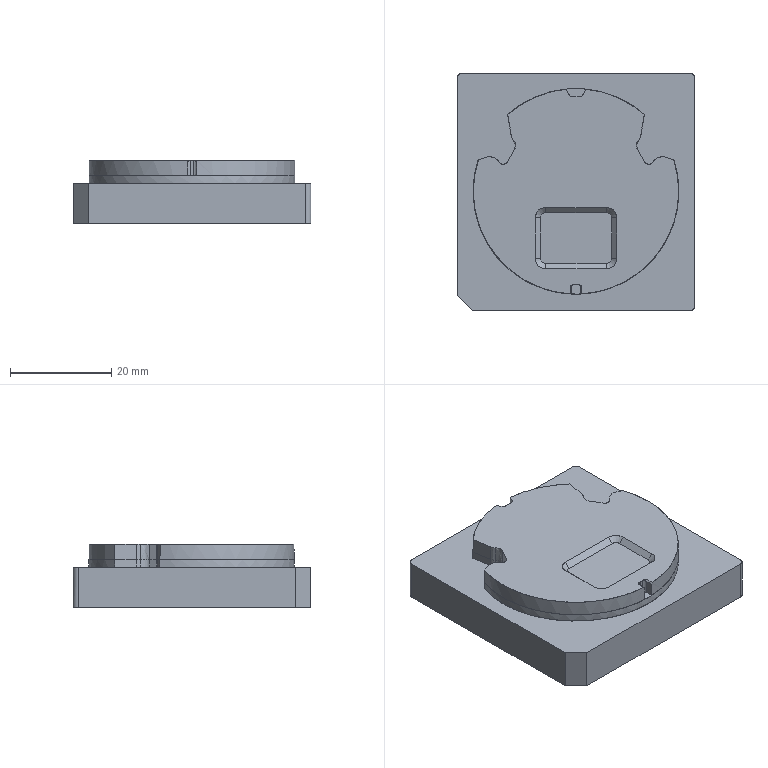NC program | PowerMill | posted with a generic post | part box 47 x 47 x 12.511 mm
Lines 1 to 1032 of 232111:
%
O0001
N104 ( POWERMILL CB  : 2026004.0)
N105 ( POST VER      : 2026.0.0.5161)
N106 ( OPTION FILE   : FANUC)
N107 ( OUTPUT WORKPLANE : WORLD)
N108 (  )
N109 ( TOOL LIST )
N110 (---------------------------------------)
N111 ( NO. | ID        | DIA.| TIP RAD|LENGTH)
N112 (---------------------------------------)
N113 (    1|D10C_1_1   |10.0 |  0.0   |67.96 )
N114 (   15|D3C_1_1    | 3.0 |  0.0   |59.56 )
N115 (   27|D1C_1_1    | 1.0 |  0.0   |59.72 )
N116 (    3|D10_1_1    |10.0 |  0.0   |67.68 )
N117 (   14|D4_1_1     | 4.0 |  0.0   |59.68 )
N118 (   12|D2_1       | 2.0 |  0.0   | 57.0 )
N119 (   12|D2_2_1     | 2.0 |  0.0   |59.68 )
N120 (    8|D1_1_1     | 1.0 |  0.0   |59.68 )
N121 (   13|TEXT_D4_1_1| 4.0 |  0.3   | 60.0 )
N122 (---------------------------------------)
N123 (  )
N124 ( NUMBER OF TOOLPATHS: 15.0 )
N125 ( ESTIMATED PROGRAM DURATION: 0 HOURS 23 MIN 32 SEC)
N126 (  )
N127 G00 G21 G80 G40 G17
N128 G90
N129 G54
N130 G53 Z0.0
N131 (---------------)
N132 ( START TOOLPATH : 精公开粗01-扫面平行-D10C )
N133 (---------------)
N134 ( TOOL NO.    :1 )
N135 ( TOOL TYPE   : ENDMILL)
N136 ( TOOL ID     : D10C_1_1)
N137 ( TOOL DIA    : 10.0 LENGTH 67.96)
N138 T1
N139 M6
N140 S8000 M03
N141 G00 G90 X0.0 Y0.0
N142 G43 Z10.2 H1
N143
N144 G05 P10000 R4
N145 X31.28 Y26.28
N146 Z1.131
N147 G01 Z-0.069 F6000.0
N148 X26.28 F10000.0
N149 X-26.28
N150 Y20.44
N151 X26.28
N152 Y14.6
N153 X-26.28
N154 Y8.76
N155 X26.28
N156 Y2.92
N157 X-26.28
N158 Y-2.92
N159 X26.28
N160 Y-8.76
N161 X-26.28
N162 Y-14.6
N163 X26.28
N164 Y-20.44
N165 X-26.28
N166 Y-26.28
N167 X26.28
N168 X31.28
N169 G00 Z10.2
N170 G05 P0
N171 (---------------)
N172 ( END TOOLPATH : 精公开粗01-扫面平行-D10C )
N173 (---------------)
N174 ( START TOOLPATH : 精公开粗01-外形偏置-D10C )
N175 (---------------)
N176 G00 X-0.0005 Y0.117 Z9.881
N177 G05 P10000 R4
N178 X-33.372 Y-5.3119
N179 Z0.7143
N180 G01 Z-0.4857 F6000.0
N181 X-32.8445 F10000.0
N182 G03 X-28.097 Y-0.5644 I0.0 J4.7475
N183 G01 Y21.0916
N184 X-23.597
N185 X-28.097
N186 Y27.217
N187 G02 X-27.097 Y28.217 I1.0 J0.0
N188 G01 X27.096
N189 G02 X28.096 Y27.217 I0.0 J-1.0
N190 G01 Y21.0926
N191 X23.596
N192 X28.096
N193 Y-21.4402
N194 X23.596
N195 X28.096
N196 Y-26.983
N197 G02 X27.096 Y-27.983 I-1.0 J0.0
N198 G01 X-27.097
N199 G02 X-28.097 Y-26.983 I0.0 J1.0
N200 G01 Y-21.4395
N201 X-23.597
N202 X-28.097
N203 Y-0.5644
N204 X-25.5545 Y-0.4862
N205 X-25.573 Y0.117
N206 X-25.524 Y1.6639
N207 X-25.3857 Y3.2107
N208 X-25.1495 Y4.7576
N209 X-24.814 Y6.3044
N210 X-24.376 Y7.8513
N211 X-24.0722 Y8.6247
N212 X-23.9767 Y8.816
N213 X-23.6102 Y9.3981
N214 X-23.2033 Y9.8987
N215 X-22.9297 Y10.1715
N216 X-22.4299 Y10.5842
N217 X-21.8609 Y10.945
N218 X-20.883 Y11.3635
N219 X-19.3362 Y11.911
N220 X-18.7817 Y12.0394
N221 G03 X-18.402 Y12.6127 I-0.1128 J0.4871
N222 G01 X-18.6516 Y14.0387
N223 X-18.7698 Y14.8121
N224 X-18.7769 Y15.5855
N225 X-18.6746 Y16.359
N226 X-18.5627 Y16.7946
N227 X-18.4454 Y17.1324
N228 X-18.0794 Y17.9058
N229 X-17.7893 Y18.3563
N230 X-17.5343 Y18.6792
N231 X-17.0159 Y19.2097
N232 X-15.8007 Y20.2261
N233 X-14.6956 Y21.0423
N234 X-13.1488 Y22.052
N235 X-11.6019 Y22.907
N236 X-10.8285 Y23.2826
N237 X-9.2816 Y23.9464
N238 X-7.7348 Y24.4956
N239 X-6.9613 Y24.7223
N240 X-5.4145 Y25.1091
N241 X-3.8676 Y25.3939
N242 X-2.3208 Y25.5875
N243 X-1.5474 Y25.5905
N244 X-0.7739 Y25.4788
N245 X-0.1565 Y25.2917
N246 X-0.0141 Y25.2702
N247 X0.1285 Y25.2902
N248 X0.7729 Y25.4782
N249 X1.5464 Y25.5905
N250 X2.3198 Y25.5876
N251 X3.8666 Y25.394
N252 X4.6401 Y25.2604
N253 X6.1869 Y24.9302
N254 X7.7338 Y24.4941
N255 X8.89 Y24.0932
N256 X10.054 Y23.6292
N257 X11.6009 Y22.9075
N258 X13.1477 Y22.0526
N259 X13.5869 Y21.7729
N260 X14.7538 Y20.9995
N261 X15.8007 Y20.2261
N262 X17.0149 Y19.2105
N263 X17.5348 Y18.6792
N264 X17.7883 Y18.357
N265 X18.079 Y17.9058
N266 X18.4452 Y17.1324
N267 X18.5617 Y16.7978
N268 X18.6743 Y16.359
N269 X18.7777 Y15.5855
N270 X18.7692 Y14.8121
N271 X18.6512 Y14.0387
N272 X18.4014 Y12.6134
N273 G03 X18.7807 Y12.04 I0.4925 J-0.0864
N274 G01 X19.3352 Y11.9112
N275 X20.882 Y11.3637
N276 X21.8607 Y10.945
N277 X22.4289 Y10.5846
N278 X22.93 Y10.1715
N279 X23.2023 Y9.8997
N280 X23.6101 Y9.3981
N281 X23.9757 Y8.8177
N282 X24.0719 Y8.6247
N283 X24.3756 Y7.8513
N284 X24.7491 Y6.5495
N285 X25.1495 Y4.7576
N286 X25.3857 Y3.2107
N287 X25.5226 Y1.6832
N288 X25.5737 Y0.117
N289 X25.5532 Y-0.6564
N290 X25.4588 Y-2.2033
N291 X25.279 Y-3.7501
N292 X24.9943 Y-5.297
N293 X24.6083 Y-6.8438
N294 X24.1164 Y-8.3907
N295 X23.5133 Y-9.9375
N296 X22.7907 Y-11.4844
N297 X21.9351 Y-13.0313
N298 X20.9325 Y-14.5781
N299 X19.7567 Y-16.125
N300 X18.5617 Y-17.4787
N301 X17.0149 Y-18.977
N302 X15.8005 Y-19.9921
N303 X14.6946 Y-20.8119
N304 X13.9212 Y-21.3373
N305 X12.2911 Y-22.3124
N306 X10.8275 Y-23.0519
N307 X9.2806 Y-23.7114
N308 X7.7338 Y-24.2559
N309 X6.9603 Y-24.4917
N310 X6.1869 Y-24.6949
N311 X4.6401 Y-25.031
N312 X3.0932 Y-25.2711
N313 X1.5981 Y-25.4061
N314 X0.7729 Y-25.4316
N315 X0.3385 Y-25.4061
N316 X0.079 Y-25.3641
N317 X-0.0005 Y-25.3577
N318 X-0.08 Y-25.364
N319 X-0.3425 Y-25.4061
N320 X-0.7739 Y-25.4317
N321 X-1.5474 Y-25.41
N322 X-3.0942 Y-25.271
N323 X-4.6411 Y-25.0308
N324 X-5.4145 Y-24.8786
N325 X-6.9613 Y-24.4916
N326 X-8.9042 Y-23.8592
N327 X-10.76 Y-23.0858
N328 X-12.2912 Y-22.3124
N329 X-13.5908 Y-21.5389
N330 X-14.6956 Y-20.8111
N331 X-15.8043 Y-19.9921
N332 X-17.0159 Y-18.9763
N333 X-18.5627 Y-17.4765
N334 X-19.7568 Y-16.125
N335 X-20.883 Y-14.6451
N336 X-21.9351 Y-13.0312
N337 X-22.7908 Y-11.4844
N338 X-23.5133 Y-9.9375
N339 X-24.1164 Y-8.3907
N340 X-24.6083 Y-6.8438
N341 X-24.9943 Y-5.297
N342 X-25.2789 Y-3.7501
N343 X-25.3768 Y-2.9767
N344 X-25.5236 Y-1.4915
N345 X-25.5545 Y-0.4862
N346 X-28.097 Y-0.5644
N347 G00 Z3.3475
N348 G01 X-33.372 Y-5.3119
N349 G00 Z0.3475
N350 G01 Z-0.8525 F6000.0
N351 X-32.8445 F10000.0
N352 G03 X-28.097 Y-0.5644 I0.0 J4.7475
N353 G01 Y0.192
N354 X-25.579 Y0.117
N355 X-25.556 Y0.8904
N356 X-25.5383 Y1.2097
N357 X-25.5239 Y1.6638
N358 X-25.4959 Y1.9769
N359 X-25.4705 Y2.4373
N360 X-25.4097 Y2.941
N361 X-25.3856 Y3.2107
N362 X-25.3454 Y3.4738
N363 X-25.2839 Y3.9841
N364 X-25.1495 Y4.7576
N365 X-24.8152 Y6.3044
N366 X-24.3812 Y7.8513
N367 X-24.0781 Y8.6247
N368 X-24.0415 Y8.6861
N369 X-23.9767 Y8.8159
N370 X-23.7377 Y9.1955
N371 X-23.6169 Y9.3981
N372 X-23.2033 Y9.9039
N373 X-22.9369 Y10.1715
N374 X-22.4299 Y10.5893
N375 X-21.8687 Y10.945
N376 X-21.6564 Y11.0543
N377 X-20.883 Y11.3681
N378 X-19.3362 Y11.9147
N379 X-18.7856 Y12.0421
N380 G03 X-18.4059 Y12.616 I-0.1127 J0.4871
N381 G01 X-18.6566 Y14.0387
N382 X-18.7732 Y14.8121
N383 X-18.7831 Y15.5855
N384 X-18.6784 Y16.359
N385 X-18.5627 Y16.807
N386 X-18.4515 Y17.1324
N387 X-18.0849 Y17.9058
N388 X-17.7893 Y18.3625
N389 X-17.5411 Y18.6792
N390 X-17.0159 Y19.2164
N391 X-16.5978 Y19.5593
N392 X-15.8006 Y20.226
N393 X-15.6435 Y20.3421
N394 X-15.469 Y20.4852
N395 X-15.0894 Y20.7514
N396 X-14.6956 Y21.0422
N397 X-14.3895 Y21.242
N398 X-13.9222 Y21.5696
N399 X-13.1488 Y22.052
N400 X-12.3753 Y22.4976
N401 X-11.9455 Y22.717
N402 X-11.6019 Y22.907
N403 X-11.02 Y23.1895
N404 X-10.8285 Y23.2873
N405 X-9.2816 Y23.9514
N406 X-7.7348 Y24.4993
N407 X-7.4357 Y24.5832
N408 X-6.9613 Y24.7223
N409 X-6.7647 Y24.7714
N410 X-6.1879 Y24.9332
N411 X-5.4145 Y25.1094
N412 X-3.8676 Y25.3966
N413 X-2.3208 Y25.5907
N414 X-1.5474 Y25.5935
N415 X-0.7739 Y25.4816
N416 X-0.1567 Y25.2943
N417 X-0.014 Y25.2728
N418 X0.1289 Y25.2929
N419 X0.7729 Y25.4813
N420 X1.5464 Y25.5934
N421 X2.3198 Y25.5908
N422 X3.8666 Y25.3967
N423 X4.6401 Y25.2637
N424 X6.1869 Y24.9335
N425 X7.7338 Y24.4987
N426 X8.399 Y24.2634
N427 X8.89 Y24.0932
N428 X8.9654 Y24.0631
N429 X9.2806 Y23.9516
N430 X9.7428 Y23.7532
N431 X10.054 Y23.6292
N432 X10.3106 Y23.5095
N433 X10.8275 Y23.2875
N434 X11.2657 Y23.0638
N435 X11.6009 Y22.9075
N436 X11.9495 Y22.7148
N437 X12.3743 Y22.4979
N438 X13.1477 Y22.0526
N439 X13.9212 Y21.5699
N440 X14.4076 Y21.2289
N441 X14.7538 Y20.9995
N442 X15.1047 Y20.7402
N443 X15.468 Y20.4855
N444 X15.637 Y20.347
N445 X15.8007 Y20.226
N446 X16.6023 Y19.5556
N447 X17.0149 Y19.2173
N448 X17.5411 Y18.6792
N449 X17.7883 Y18.364
N450 X18.0851 Y17.9058
N451 X18.4518 Y17.1324
N452 X18.4871 Y17.0119
N453 X18.5617 Y16.7978
N454 X18.6449 Y16.4731
N455 X18.6784 Y16.359
N456 X18.7831 Y15.5855
N457 X18.7732 Y14.8121
N458 X18.7317 Y14.5663
N459 X18.6512 Y14.0387
N460 X18.4118 Y12.6725
N461 X18.4018 Y12.6135
N462 G03 X18.782 Y12.0431 I0.493 J-0.0833
N463 G01 X19.3352 Y11.915
N464 X20.882 Y11.3684
N465 X21.6554 Y11.0548
N466 X21.8687 Y10.945
N467 X22.4289 Y10.59
N468 X22.9369 Y10.1715
N469 X23.2023 Y9.905
N470 X23.6169 Y9.3981
N471 X23.7404 Y9.1912
N472 X23.9757 Y8.8177
N473 X24.0382 Y8.6922
N474 X24.0785 Y8.6247
N475 X24.3815 Y7.8513
N476 X24.7491 Y6.5496
N477 X24.9892 Y5.531
N478 X25.0619 Y5.1496
N479 X25.1495 Y4.7575
N480 X25.2012 Y4.419
N481 X25.2841 Y3.9841
N482 X25.3857 Y3.2107
N483 X25.5243 Y1.6639
N484 X25.5788 Y0.117
N485 X25.5542 Y-0.6192
N486 X25.5532 Y-0.6564
N487 X25.5526 Y-0.6658
N488 X25.5226 Y-1.5633
N489 X25.466 Y-2.0844
N490 X25.4588 Y-2.2033
N491 X25.3741 Y-2.932
N492 X25.2853 Y-3.7501
N493 X24.9944 Y-5.297
N494 X24.8102 Y-6.0704
N495 X24.7228 Y-6.3847
N496 X24.6083 Y-6.8438
N497 X24.5036 Y-7.1729
N498 X24.38 Y-7.6173
N499 X24.2005 Y-8.1259
N500 X24.1163 Y-8.3907
N501 X24.0191 Y-8.6401
N502 X23.8342 Y-9.1641
N503 X23.5133 Y-9.9375
N504 X22.7908 Y-11.4844
N505 X21.9378 Y-13.0313
N506 X20.9365 Y-14.5781
N507 X19.7609 Y-16.125
N508 X18.5617 Y-17.4834
N509 X17.0149 Y-18.9812
N510 X16.7046 Y-19.2363
N511 X15.8005 Y-19.992
N512 X15.6464 Y-20.1063
N513 X15.468 Y-20.2529
N514 X15.0835 Y-20.5235
N515 X14.6946 Y-20.8118
N516 X14.0981 Y-21.2171
N517 X13.9212 Y-21.3416
N518 X12.2978 Y-22.3124
N519 X10.7621 Y-23.0858
N520 X10.062 Y-23.3782
N521 X9.2806 Y-23.7113
N522 X9.1771 Y-23.7478
N523 X8.9102 Y-23.8592
N524 X8.215 Y-24.0864
N525 X7.7337 Y-24.2558
N526 X7.1786 Y-24.4251
N527 X6.9603 Y-24.4964
N528 X6.1869 Y-24.6949
N529 X4.6401 Y-25.0317
N530 X3.0932 Y-25.275
N531 X1.6012 Y-25.4061
N532 X0.7729 Y-25.4398
N533 X0.5801 Y-25.4202
N534 X0.3385 Y-25.406
N535 X0.1663 Y-25.3782
N536 X-0.0005 Y-25.3612
N537 X-0.1715 Y-25.3786
N538 X-0.3425 Y-25.406
N539 X-0.5797 Y-25.4201
N540 X-0.7739 Y-25.4399
N541 X-1.5474 Y-25.4104
N542 X-3.0942 Y-25.2749
N543 X-3.8676 Y-25.1586
N544 X-4.1866 Y-25.1014
N545 X-4.6411 Y-25.0308
N546 X-5.2767 Y-24.9057
N547 X-5.4145 Y-24.881
N548 X-6.9613 Y-24.4961
N549 X-8.9129 Y-23.8592
N550 X-10.7676 Y-23.0858
N551 X-12.2979 Y-22.3124
N552 X-13.9222 Y-21.3411
N553 X-14.3771 Y-21.0209
N554 X-14.6956 Y-20.8111
N555 X-15.1068 Y-20.5073
N556 X-15.469 Y-20.2524
N557 X-15.6204 Y-20.1279
N558 X-15.8043 Y-19.992
N559 X-16.7519 Y-19.1976
N560 X-17.0159 Y-18.9805
N561 X-18.3773 Y-17.6718
N562 X-18.4829 Y-17.5538
N563 X-18.5627 Y-17.4764
N564 X-19.4146 Y-16.5122
N565 X-19.761 Y-16.125
N566 X-20.9364 Y-14.5781
N567 X-21.938 Y-13.0312
N568 X-22.7908 Y-11.4844
N569 X-23.1675 Y-10.711
N570 X-23.3592 Y-10.2674
N571 X-23.5133 Y-9.9375
N572 X-23.6194 Y-9.6654
N573 X-23.8361 Y-9.1641
N574 X-24.032 Y-8.6071
N575 X-24.1164 Y-8.3907
N576 X-24.1939 Y-8.1467
N577 X-24.3802 Y-7.6173
N578 X-24.6083 Y-6.8438
N579 X-24.9962 Y-5.297
N580 X-25.2854 Y-3.7501
N581 X-25.3256 Y-3.3813
N582 X-25.3768 Y-2.9767
N583 X-25.4478 Y-2.258
N584 X-25.5236 Y-1.5616
N585 X-25.579 Y0.117
N586 X-28.097 Y0.192
N587 Y21.0993
N588 X-23.597
N589 X-28.097
N590 Y27.217
N591 G02 X-27.097 Y28.217 I1.0 J0.0
N592 G01 X27.096
N593 G02 X28.096 Y27.217 I0.0 J-1.0
N594 G01 Y21.1009
N595 X23.596
N596 X28.096
N597 Y-21.4426
N598 X23.596
N599 X28.096
N600 Y-26.983
N601 G02 X27.096 Y-27.983 I-1.0 J0.0
N602 G01 X-27.097
N603 G02 X-28.097 Y-26.983 I0.0 J1.0
N604 G01 Y-21.4391
N605 X-23.597
N606 X-28.097
N607 Y-0.5644
N608 G00 Z2.9808
N609 G01 X-33.372 Y-5.3119
N610 G00 Z-0.0192
N611 G01 Z-1.2192 F6000.0
N612 X-32.8445 F10000.0
N613 G03 X-28.097 Y-0.5644 I0.0 J4.7475
N614 G01 Y-0.1852
N615 X-25.5749 Y-0.1
N616 X-25.5822 Y0.117
N617 X-25.5589 Y0.8904
N618 X-25.5342 Y1.3394
N619 X-25.5239 Y1.6638
N620 X-25.5039 Y1.8867
N621 X-25.4735 Y2.4373
N622 X-25.4 Y3.0495
N623 X-25.3856 Y3.2107
N624 X-25.3622 Y3.3634
N625 X-25.2876 Y3.9841
N626 X-25.1495 Y4.7576
N627 X-24.8185 Y6.3044
N628 X-24.3854 Y7.8513
N629 X-24.0823 Y8.6247
N630 X-24.0195 Y8.7301
N631 X-23.9766 Y8.8159
N632 X-23.8198 Y9.065
N633 X-23.6212 Y9.3981
N634 X-23.2033 Y9.9091
N635 X-22.9421 Y10.1715
N636 X-22.4299 Y10.594
N637 X-21.8758 Y10.945
N638 X-21.6564 Y11.0589
N639 X-20.883 Y11.3724
N640 X-19.3362 Y11.9181
N641 X-18.7858 Y12.0454
N642 G03 X-18.4013 Y12.5848 I-0.1128 J0.4872
N643 G01 X-18.4033 Y12.6005
N644 X-18.4058 Y12.616
N645 X-18.6566 Y14.0387
N646 X-18.7449 Y14.6246
N647 X-18.7766 Y14.8121
N648 X-18.7866 Y15.5855
N649 X-18.6821 Y16.359
N650 X-18.6502 Y16.4681
N651 X-18.5627 Y16.8069
N652 X-18.4812 Y17.0454
N653 X-18.4558 Y17.1324
N654 X-18.0896 Y17.9058
N655 X-17.7893 Y18.3686
N656 X-17.5456 Y18.6792
N657 X-17.0159 Y19.2207
N658 X-16.3395 Y19.7753
N659 X-15.8006 Y20.226
N660 X-15.6923 Y20.306
N661 X-15.469 Y20.4891
N662 X-14.986 Y20.8277
N663 X-14.6955 Y21.0422
N664 X-14.4686 Y21.1903
N665 X-13.9222 Y21.5733
N666 X-13.7649 Y21.6677
N667 X-13.1487 Y22.052
N668 X-12.5279 Y22.4097
N669 X-12.3753 Y22.5012
N670 X-11.8606 Y22.7639
N671 X-11.6019 Y22.9069
N672 X-11.1617 Y23.1207
N673 X-10.8285 Y23.2908
N674 X-9.2816 Y23.9557
N675 X-7.7348 Y24.5027
N676 X-7.1663 Y24.6621
N677 X-6.9613 Y24.7222
N678 X-6.8761 Y24.7435
N679 X-6.1879 Y24.9365
N680 X-5.4145 Y25.1099
N681 X-3.8676 Y25.3996
N682 X-2.3208 Y25.5939
N683 X-1.5474 Y25.5965
N684 X-0.7739 Y25.4843
N685 X-0.1568 Y25.2969
N686 X-0.014 Y25.2754
N687 X0.129 Y25.2955
N688 X0.7729 Y25.4841
N689 X1.5464 Y25.5964
N690 X2.3198 Y25.594
N691 X3.8666 Y25.3998
N692 X4.6401 Y25.267
N693 X6.1869 Y24.9368
N694 X7.7338 Y24.503
N695 X9.2806 Y23.956
N696 X9.8747 Y23.7006
N697 X10.054 Y23.6291
N698 X10.2065 Y23.558
N699 X10.8275 Y23.291
N700 X11.3471 Y23.0258
N701 X11.6009 Y22.9074
N702 X11.8643 Y22.7618
N703 X12.3743 Y22.5015
N704 X12.525 Y22.4111
N705 X13.1477 Y22.0526
N706 X13.7639 Y21.668
N707 X13.9212 Y21.5737
N708 X14.5093 Y21.1615
N709 X14.7538 Y20.9994
N710 X15.0001 Y20.8174
N711 X15.468 Y20.4895
N712 X15.6869 Y20.31
N713 X15.8007 Y20.226
N714 X16.3492 Y19.7672
N715 X17.0149 Y19.2216
N716 X17.5456 Y18.6792
N717 X17.7883 Y18.3699
N718 X18.0896 Y17.9058
N719 X18.4558 Y17.1324
N720 X18.5117 Y16.9412
N721 X18.5616 Y16.7978
N722 X18.6181 Y16.5778
N723 X18.6821 Y16.359
N724 X18.7866 Y15.5855
N725 X18.7766 Y14.8121
N726 X18.6609 Y14.0387
N727 X18.4097 Y12.6191
N728 G03 X18.7891 Y12.045 I0.4924 J-0.0871
N729 G01 X19.3352 Y11.9183
N730 X20.882 Y11.3728
N731 X21.6554 Y11.0594
N732 X21.8758 Y10.945
N733 X22.4289 Y10.5947
N734 X22.9421 Y10.1715
N735 X23.2023 Y9.9102
N736 X23.6212 Y9.3981
N737 X23.8196 Y9.0654
N738 X23.9756 Y8.8176
N739 X24.0184 Y8.7319
N740 X24.0823 Y8.6247
N741 X24.3854 Y7.8513
N742 X24.8187 Y6.3044
N743 X24.9924 Y5.531
N744 X25.0843 Y5.049
N745 X25.1494 Y4.7575
N746 X25.1879 Y4.5056
N747 X25.2873 Y3.9841
N748 X25.3222 Y3.694
N749 X25.3857 Y3.2107
N750 X25.4017 Y3.0319
N751 X25.4731 Y2.4373
N752 X25.5226 Y1.733
N753 X25.582 Y0.117
N754 X25.5226 Y-1.6306
N755 X25.2885 Y-3.7501
N756 X24.9975 Y-5.297
N757 X24.8136 Y-6.0704
N758 X24.6909 Y-6.5123
N759 X24.6082 Y-6.8438
N760 X24.5355 Y-7.0724
N761 X24.3843 Y-7.6173
N762 X24.164 Y-8.2405
N763 X24.1163 Y-8.3907
N764 X24.0593 Y-8.5368
N765 X23.8376 Y-9.1641
N766 X23.5134 Y-9.9375
N767 X22.7924 Y-11.4844
N768 X21.9416 Y-13.0313
N769 X20.9404 Y-14.5781
N770 X19.7651 Y-16.125
N771 X18.5617 Y-17.4881
N772 X17.0149 Y-18.9854
N773 X16.4021 Y-19.4891
N774 X15.8004 Y-19.992
N775 X15.6964 Y-20.0691
N776 X15.468 Y-20.2568
N777 X14.9782 Y-20.6015
N778 X14.6945 Y-20.8118
N779 X14.2563 Y-21.1095
N780 X13.9212 Y-21.3453
N781 X12.3743 Y-22.2741
N782 X10.7693 Y-23.0858
N783 X9.6701 Y-23.5452
N784 X9.2806 Y-23.7113
N785 X9.2312 Y-23.7287
N786 X8.9188 Y-23.8592
N787 X8.0749 Y-24.1357
N788 X7.7337 Y-24.2558
N789 X7.3656 Y-24.368
N790 X6.9603 Y-24.5008
N791 X6.6172 Y-24.5845
N792 X6.1869 Y-24.6949
N793 X5.9759 Y-24.7408
N794 X5.4135 Y-24.878
N795 X4.6401 Y-25.0349
N796 X3.0932 Y-25.2783
N797 X1.6083 Y-25.4061
N798 X0.7729 Y-25.4433
N799 X0.4947 Y-25.4152
N800 X0.3385 Y-25.406
N801 X0.2299 Y-25.3884
N802 X-0.0005 Y-25.3651
N803 X-0.2366 Y-25.389
N804 X-0.3425 Y-25.406
N805 X-0.4931 Y-25.4149
N806 X-0.7739 Y-25.4433
N807 X-1.5474 Y-25.4111
N808 X-3.0942 Y-25.2781
N809 X-3.8676 Y-25.1606
N810 X-4.2722 Y-25.088
N811 X-4.641 Y-25.0307
N812 X-5.1516 Y-24.9303
N813 X-5.4145 Y-24.8831
N814 X-6.9613 Y-24.5005
N815 X-8.9217 Y-23.8592
N816 X-10.7751 Y-23.0858
N817 X-12.3046 Y-22.3124
N818 X-13.9222 Y-21.3448
N819 X-14.4634 Y-20.9639
N820 X-14.6955 Y-20.811
N821 X-14.9936 Y-20.5908
N822 X-15.469 Y-20.2563
N823 X-15.6687 Y-20.0921
N824 X-15.8043 Y-19.992
N825 X-16.4937 Y-19.414
N826 X-17.0159 Y-18.9848
N827 X-18.3819 Y-17.6718
N828 X-18.5176 Y-17.5201
N829 X-18.5627 Y-17.4764
N830 X-19.0561 Y-16.918
N831 X-19.7652 Y-16.125
N832 X-20.9406 Y-14.5781
N833 X-21.9418 Y-13.0312
N834 X-22.7919 Y-11.4844
N835 X-23.1704 Y-10.711
N836 X-23.3998 Y-10.1803
N837 X-23.5133 Y-9.9375
N838 X-23.5907 Y-9.7389
N839 X-23.8392 Y-9.1641
N840 X-24.07 Y-8.5096
N841 X-24.1163 Y-8.3907
N842 X-24.1571 Y-8.2623
N843 X-24.3845 Y-7.6173
N844 X-24.6083 Y-6.8438
N845 X-24.9991 Y-5.297
N846 X-25.2887 Y-3.7501
N847 X-25.3549 Y-3.149
N848 X-25.3767 Y-2.9767
N849 X-25.4012 Y-2.7294
N850 X-25.5236 Y-1.6189
N851 X-25.5749 Y-0.1
N852 X-28.097 Y-0.1852
N853 Y21.1046
N854 X-23.597
N855 X-28.097
N856 Y27.217
N857 G02 X-27.097 Y28.217 I1.0 J0.0
N858 G01 X27.096
N859 G02 X28.096 Y27.217 I0.0 J-1.0
N860 G01 Y21.1058
N861 X23.596
N862 X28.096
N863 Y-21.4449
N864 X23.596
N865 X28.096
N866 Y-26.983
N867 G02 X27.096 Y-27.983 I-1.0 J0.0
N868 G01 X-27.097
N869 G02 X-28.097 Y-26.983 I0.0 J1.0
N870 G01 Y-21.4415
N871 X-23.597
N872 X-28.097
N873 Y-0.5644
N874 G00 Z2.614
N875 G01 X-33.372 Y-5.3119
N876 G00 Z-0.386
N877 G01 Z-1.586 F6000.0
N878 X-32.8445 F10000.0
N879 G03 X-28.097 Y-0.5644 I0.0 J4.7475
N880 G01 Y-0.1936
N881 X-25.5777 Y-0.1064
N882 X-25.5854 Y0.117
N883 X-25.5619 Y0.8904
N884 X-25.53 Y1.4697
N885 X-25.5238 Y1.6638
N886 X-25.5119 Y1.7967
N887 X-25.4766 Y2.4373
N888 X-25.3907 Y3.153
N889 X-25.3855 Y3.2107
N890 X-25.3772 Y3.2649
N891 X-25.2909 Y3.9841
N892 X-25.1496 Y4.7576
N893 X-24.8218 Y6.3044
N894 X-24.3888 Y7.8513
N895 X-24.0861 Y8.6247
N896 X-23.9992 Y8.7705
N897 X-23.9766 Y8.8159
N898 X-23.8961 Y8.9437
N899 X-23.6256 Y9.3981
N900 X-23.2033 Y9.9144
N901 X-22.9473 Y10.1715
N902 X-22.4299 Y10.5983
N903 X-21.8828 Y10.945
N904 X-21.6564 Y11.0626
N905 X-20.883 Y11.3759
N906 X-19.3362 Y11.9214
N907 X-18.7929 Y12.0472
N908 G03 X-18.4134 Y12.6214 I-0.1129 J0.4871
N909 G01 X-18.6641 Y14.0387
N910 X-18.7799 Y14.8121
N911 X-18.7901 Y15.5855
N912 X-18.6858 Y16.359
N913 X-18.6215 Y16.5789
N914 X-18.5626 Y16.8069
N915 X-18.5085 Y16.9653
N916 X-18.4597 Y17.1324
N917 X-18.0937 Y17.9058
N918 X-17.7893 Y18.3745
N919 X-17.55 Y18.6792
N920 X-17.0159 Y19.2249
N921 X-16.0895 Y19.9844
N922 X-15.8006 Y20.226
N923 X-15.7414 Y20.2696
N924 X-15.469 Y20.493
N925 X-14.8832 Y20.9035
N926 X-14.6955 Y21.0421
N927 X-14.5481 Y21.1384
N928 X-13.9222 Y21.577
N929 X-13.6088 Y21.765
N930 X-13.1487 Y22.052
N931 X-12.6817 Y22.321
N932 X-12.3753 Y22.5047
N933 X-11.776 Y22.8106
N934 X-11.6018 Y22.9069
N935 X-11.3042 Y23.0514
N936 X-10.8285 Y23.2942
N937 X-9.2816 Y23.9591
N938 X-7.7348 Y24.5061
N939 X-6.1879 Y24.9399
N940 X-5.4145 Y25.1132
N941 X-3.8676 Y25.4029
N942 X-2.3208 Y25.5971
N943 X-1.5474 Y25.5995
N944 X-0.7739 Y25.4871
N945 X-0.1569 Y25.2995
N946 X-0.014 Y25.2779
N947 X0.1292 Y25.2981
N948 X0.7729 Y25.4868
N949 X1.5464 Y25.5994
N950 X2.3198 Y25.5972
N951 X3.8666 Y25.403
N952 X4.6401 Y25.2703
N953 X6.1869 Y24.9401
N954 X7.7338 Y24.5064
N955 X9.2806 Y23.9594
N956 X9.9868 Y23.6559
N957 X10.054 Y23.6291
N958 X10.111 Y23.6025
N959 X10.8275 Y23.2945
N960 X11.4289 Y22.9876
N961 X11.6008 Y22.9074
N962 X11.7787 Y22.8091
N963 X12.3743 Y22.5051
N964 X12.6789 Y22.3225
N965 X13.1477 Y22.0525
N966 X13.608 Y21.7653
N967 X13.9212 Y21.5775
N968 X14.6115 Y21.0937
N969 X14.7537 Y20.9994
N970 X14.8962 Y20.8942
N971 X15.468 Y20.4934
N972 X15.7371 Y20.2729
N973 X15.8006 Y20.226
N974 X16.1027 Y19.9733
N975 X17.0149 Y19.2258
N976 X17.55 Y18.6792
N977 X17.7883 Y18.3759
N978 X18.0937 Y17.9058
N979 X18.4597 Y17.1324
N980 X18.5361 Y16.8711
N981 X18.5616 Y16.7978
N982 X18.5908 Y16.684
N983 X18.6858 Y16.359
N984 X18.7901 Y15.5855
N985 X18.7799 Y14.8121
N986 X18.6641 Y14.0387
N987 X18.4134 Y12.6218
N988 G03 X18.7927 Y12.0476 I0.4924 J-0.0871
N989 G01 X19.3352 Y11.9216
N990 X20.882 Y11.3762
N991 X21.6554 Y11.0631
N992 X21.8828 Y10.945
N993 X22.4289 Y10.5991
N994 X22.9473 Y10.1715
N995 X23.2023 Y9.9154
N996 X23.6256 Y9.3981
N997 X23.9757 Y8.8395
N998 X24.0861 Y8.6247
N999 X24.3887 Y7.8513
N1000 X24.822 Y6.3044
N1001 X24.9957 Y5.531
N1002 X25.1067 Y4.9485
N1003 X25.1494 Y4.7575
N1004 X25.1746 Y4.5923
N1005 X25.2905 Y3.9841
N1006 X25.3602 Y3.4041
N1007 X25.3856 Y3.2107
N1008 X25.392 Y3.1391
N1009 X25.4763 Y2.4373
N1010 X25.5226 Y1.8062
N1011 X25.5852 Y0.117
N1012 X25.5226 Y-1.6842
N1013 X25.2918 Y-3.7501
N1014 X25.0008 Y-5.297
N1015 X24.8169 Y-6.0704
N1016 X24.6606 Y-6.6335
N1017 X24.6082 Y-6.8438
N1018 X24.5622 Y-6.9884
N1019 X24.3877 Y-7.6173
N1020 X24.1331 Y-8.3376
N1021 X24.1162 Y-8.3906
N1022 X24.0961 Y-8.4422
N1023 X23.841 Y-9.1641
N1024 X23.5152 Y-9.9375
N1025 X22.796 Y-11.4844
N1026 X21.9454 Y-13.0313
N1027 X20.9444 Y-14.5781
N1028 X19.7693 Y-16.125
N1029 X18.5617 Y-17.4928
N1030 X17.0149 Y-18.9896
N1031 X16.1071 Y-19.7357
N1032 X15.8004 Y-19.992
N1033 X15.7466 Y-20.0318
N1034 X15.468 Y-20.2608
N1035 X14.8735 Y-20.6791
N1036 X14.6945 Y-20.8118
N1037 X14.4159 Y-21.001
N1038 X13.9212 Y-21.3491
N1039 X12.3743 Y-22.2777
N1040 X10.7764 Y-23.0858
N1041 X8.9274 Y-23.8592
N1042 X7.9467 Y-24.1807
N1043 X7.7337 Y-24.2557
N1044 X7.5088 Y-24.3243
N1045 X6.9603 Y-24.5041
N1046 X6.3548 Y-24.6518
N1047 X6.1869 Y-24.6949
N1048 X6.1043 Y-24.7128
N1049 X5.4135 Y-24.8813
N1050 X4.6401 Y-25.0382
N1051 X3.0932 Y-25.2815
N1052 X1.6456 Y-25.4061
N1053 X0.7729 Y-25.4467
N1054 X0.4068 Y-25.4099
N1055 X0.3385 Y-25.4059
N1056 X0.2923 Y-25.3984
N1057 X-0.0005 Y-25.369
N1058 X-0.3004 Y-25.3992
N1059 X-0.3426 Y-25.4059
N1060 X-0.404 Y-25.4096
N1061 X-0.7739 Y-25.4467
N1062 X-1.5474 Y-25.4142
N1063 X-3.0942 Y-25.2814
N1064 X-3.8676 Y-25.1626
N1065 X-4.3577 Y-25.0747
N1066 X-4.641 Y-25.0307
N1067 X-5.0305 Y-24.954
N1068 X-5.4145 Y-24.8852
N1069 X-6.9613 Y-24.5038
N1070 X-8.9304 Y-23.8592
N1071 X-10.7821 Y-23.0858
N1072 X-12.3114 Y-22.3124
N1073 X-13.9222 Y-21.3486
N1074 X-14.5502 Y-20.9067
N1075 X-14.6955 Y-20.811
N1076 X-14.8812 Y-20.6738
N1077 X-15.469 Y-20.2602
N1078 X-15.7172 Y-20.0562
N1079 X-15.8042 Y-19.992
N1080 X-16.2412 Y-19.6256
N1081 X-17.0159 Y-18.989
N1082 X-18.3865 Y-17.6718
N1083 X-18.5522 Y-17.4865
N1084 X-18.5626 Y-17.4764
N1085 X-18.6799 Y-17.3436
N1086 X-19.7694 Y-16.125
N1087 X-20.9445 Y-14.5781
N1088 X-21.9456 Y-13.0312
N1089 X-22.7955 Y-11.4844
N1090 X-23.1733 Y-10.711
N1091 X-23.4408 Y-10.0925
N1092 X-23.5132 Y-9.9375
N1093 X-23.5623 Y-9.8116
N1094 X-23.8423 Y-9.1641
N1095 X-24.1045 Y-8.421
N1096 X-24.1163 Y-8.3906
N1097 X-24.1266 Y-8.3582
N1098 X-24.3879 Y-7.6173
N1099 X-24.6084 Y-6.8438
N1100 X-25.002 Y-5.297
N1101 X-25.2919 Y-3.7501
N1102 X-25.5236 Y-1.6706
N1103 X-25.5777 Y-0.1064
N1104 X-28.097 Y-0.1936
N1105 Y21.1095
N1106 X-23.597
N1107 X-28.097
N1108 Y27.217
N1109 G02 X-27.097 Y28.217 I1.0 J0.0
N1110 G01 X27.096
N1111 G02 X28.096 Y27.217 I0.0 J-1.0
N1112 G01 Y21.1107
N1113 X23.596
N1114 X28.096
N1115 Y-21.4473
N1116 X23.596
N1117 X28.096
N1118 Y-26.983
N1119 G02 X27.096 Y-27.983 I-1.0 J0.0
N1120 G01 X-27.097
N1121 G02 X-28.097 Y-26.983 I0.0 J1.0
N1122 G01 Y-21.4439
N1123 X-23.597
N1124 X-28.097
N1125 Y-0.5644
N1126 G00 Z2.2473
N1127 G01 X-33.372 Y-5.3119
N1128 G00 Z-0.7527
N1129 G01 Z-1.9527 F6000.0